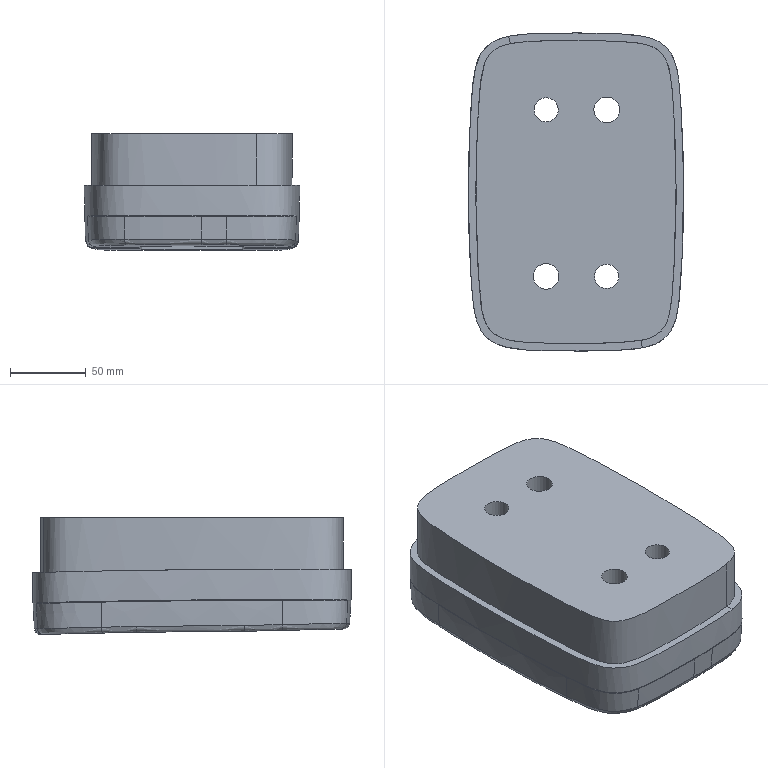Part | NX | features solid 2 | 1 solid | 61 faces | box 142.217 x 210.106 x 77.193 mm | volume 1864734 mm3 | spline 48 | cylinder 8 | plane 5 | commonest cylinder face diameters 17 x4 16 x2 26 x2